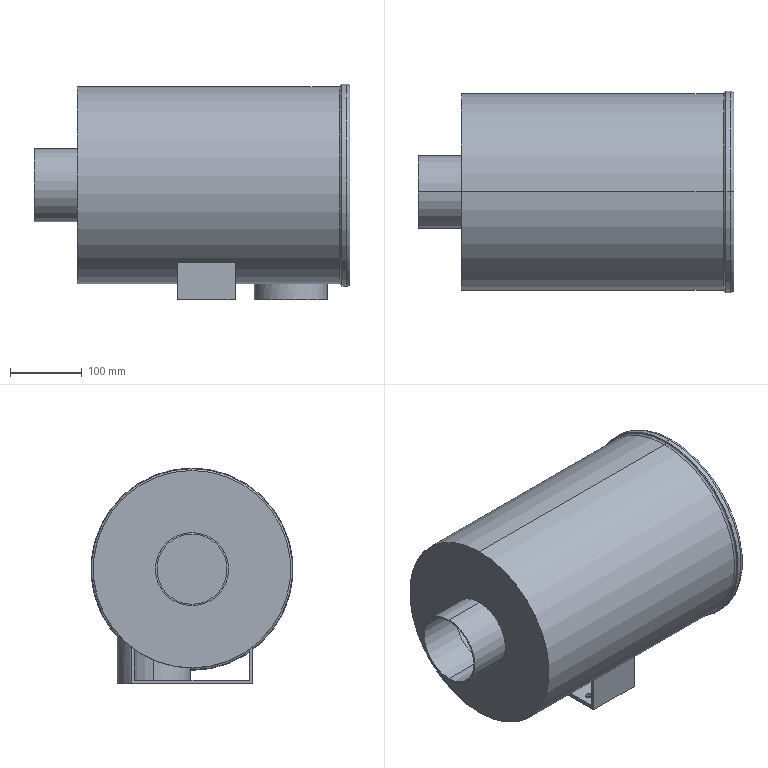Part | SolidWorks | features BaseBody 2 | 2 solids | 44 faces | box 440 x 282 x 301 mm | volume 1801894 mm3 | cylinder 24 | plane 14 | torus 6 | commonest cylinder face diameters 10 x8 98 x4 102 x4 275 x4 270 x2 282 x2